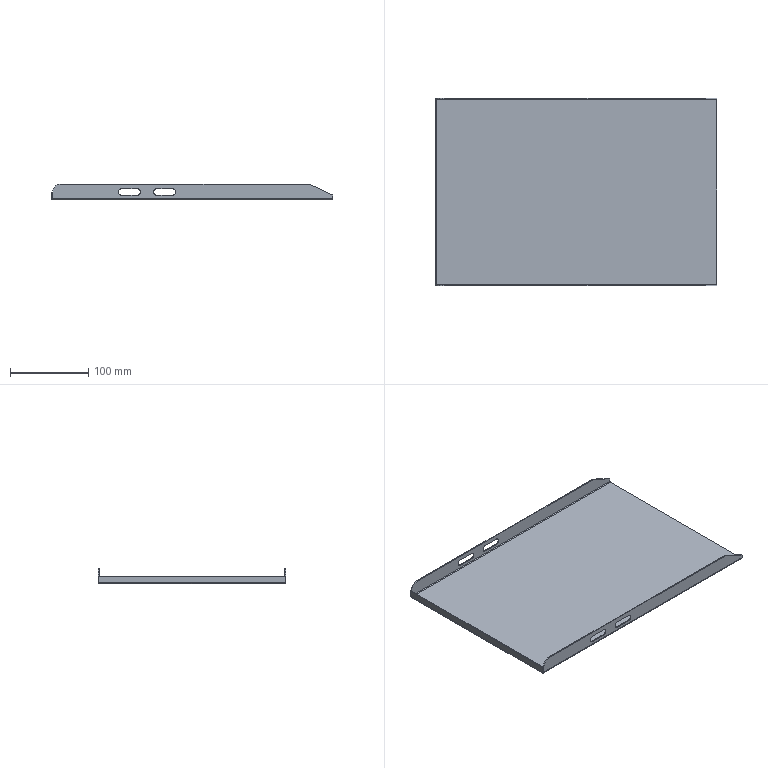Part | 1 solid | 52 faces | box 360 x 240 x 20 mm | volume 120091 mm3 | plane 36 | cylinder 16 | commonest cylinder face diameters 8.4 x8 1.473 x3 3.873 x3 20 x2
STEP:
#1=CARTESIAN_POINT('',(-178.063,120.,0.));
#2=VERTEX_POINT('',#1);
#3=CARTESIAN_POINT('',(-178.063,119.854,0.));
#4=VERTEX_POINT('',#3);
#5=CARTESIAN_POINT('',(-178.063,120.,0.));
#6=DIRECTION('',(0.,-1.,0.));
#7=VECTOR('',#6,1000.);
#8=LINE('',#5,#7);
#9=EDGE_CURVE('',#2,#4,#8,.T.);
#10=ORIENTED_EDGE('',*,*,#9,.T.);
#11=CARTESIAN_POINT('',(-178.063,118.063,-1.2));
#12=VERTEX_POINT('',#11);
#13=CARTESIAN_POINT('',(-178.063,118.063,0.7366));
#14=DIRECTION('',(-1.,0.,0.));
#15=DIRECTION('',(0.,0.,1.));
#16=AXIS2_PLACEMENT_3D('',#13,#14,#15);
#17=CIRCLE('',#16,1.937);
#18=EDGE_CURVE('',#4,#12,#17,.T.);
#19=ORIENTED_EDGE('',*,*,#18,.T.);
#20=CARTESIAN_POINT('',(-178.063,120.,-1.2));
#21=VERTEX_POINT('',#20);
#22=CARTESIAN_POINT('',(-178.063,-120.,-1.2));
#23=DIRECTION('',(0.,-1.,0.));
#24=VECTOR('',#23,1000.);
#25=LINE('',#22,#24);
#26=EDGE_CURVE('',#21,#12,#25,.T.);
#27=ORIENTED_EDGE('',*,*,#26,.F.);
#28=CARTESIAN_POINT('',(-178.063,120.,0.));
#29=DIRECTION('',(0.,0.,-1.));
#30=VECTOR('',#29,1000.);
#31=LINE('',#28,#30);
#32=EDGE_CURVE('',#2,#21,#31,.T.);
#33=ORIENTED_EDGE('',*,*,#32,.F.);
#34=EDGE_LOOP('',(#10,#19,#27,#33));
#35=FACE_OUTER_BOUND('',#34,.T.);
#36=CARTESIAN_POINT('',(-178.063,120.,0.));
#37=DIRECTION('',(1.,0.,0.));
#38=DIRECTION('',(0.,0.,-1.));
#39=AXIS2_PLACEMENT_3D('',#36,#37,#38);
#40=PLANE('',#39);
#41=ADVANCED_FACE('',(#35),#40,.T.);
#42=CARTESIAN_POINT('',(-178.063,-120.,-1.2));
#43=VERTEX_POINT('',#42);
#44=CARTESIAN_POINT('',(-178.063,-118.063,-1.2));
#45=VERTEX_POINT('',#44);
#46=CARTESIAN_POINT('',(-178.063,-120.,-1.2));
#47=DIRECTION('',(0.,1.,0.));
#48=VECTOR('',#47,1000.);
#49=LINE('',#46,#48);
#50=EDGE_CURVE('',#43,#45,#49,.T.);
#51=ORIENTED_EDGE('',*,*,#50,.T.);
#52=CARTESIAN_POINT('',(-178.063,-119.854,0.));
#53=VERTEX_POINT('',#52);
#54=CARTESIAN_POINT('',(-178.063,-118.063,0.7366));
#55=DIRECTION('',(-1.,0.,0.));
#56=DIRECTION('',(0.,0.,-1.));
#57=AXIS2_PLACEMENT_3D('',#54,#55,#56);
#58=CIRCLE('',#57,1.937);
#59=EDGE_CURVE('',#45,#53,#58,.T.);
#60=ORIENTED_EDGE('',*,*,#59,.T.);
#61=CARTESIAN_POINT('',(-178.063,-120.,0.));
#62=VERTEX_POINT('',#61);
#63=CARTESIAN_POINT('',(-178.063,-120.,0.));
#64=DIRECTION('',(0.,1.,0.));
#65=VECTOR('',#64,1000.);
#66=LINE('',#63,#65);
#67=EDGE_CURVE('',#62,#53,#66,.T.);
#68=ORIENTED_EDGE('',*,*,#67,.F.);
#69=CARTESIAN_POINT('',(-178.063,-120.,0.));
#70=DIRECTION('',(0.,0.,-1.));
#71=VECTOR('',#70,1000.);
#72=LINE('',#69,#71);
#73=EDGE_CURVE('',#62,#43,#72,.T.);
#74=ORIENTED_EDGE('',*,*,#73,.T.);
#75=EDGE_LOOP('',(#51,#60,#68,#74));
#76=FACE_OUTER_BOUND('',#75,.T.);
#77=CARTESIAN_POINT('',(-178.063,-118.063,0.));
#78=DIRECTION('',(1.,0.,0.));
#79=DIRECTION('',(0.,0.,-1.));
#80=AXIS2_PLACEMENT_3D('',#77,#78,#79);
#81=PLANE('',#80);
#82=ADVANCED_FACE('',(#76),#81,.T.);
#83=CARTESIAN_POINT('',(-178.063,-120.,-1.2));
#84=DIRECTION('',(0.,1.,0.));
#85=VECTOR('',#84,1000.);
#86=LINE('',#83,#85);
#87=EDGE_CURVE('',#45,#12,#86,.T.);
#88=ORIENTED_EDGE('',*,*,#87,.T.);
#89=CARTESIAN_POINT('',(180.,118.063,-1.2));
#90=VERTEX_POINT('',#89);
#91=CARTESIAN_POINT('',(-178.063,118.063,-1.2));
#92=DIRECTION('',(1.,0.,0.));
#93=VECTOR('',#92,1000.);
#94=LINE('',#91,#93);
#95=EDGE_CURVE('',#12,#90,#94,.T.);
#96=ORIENTED_EDGE('',*,*,#95,.T.);
#97=CARTESIAN_POINT('',(180.,-118.063,-1.2));
#98=VERTEX_POINT('',#97);
#99=CARTESIAN_POINT('',(180.,-120.,-1.2));
#100=DIRECTION('',(0.,1.,0.));
#101=VECTOR('',#100,1000.);
#102=LINE('',#99,#101);
#103=EDGE_CURVE('',#98,#90,#102,.T.);
#104=ORIENTED_EDGE('',*,*,#103,.F.);
#105=CARTESIAN_POINT('',(180.,-118.063,-1.2));
#106=DIRECTION('',(-1.,0.,0.));
#107=VECTOR('',#106,1000.);
#108=LINE('',#105,#107);
#109=EDGE_CURVE('',#98,#45,#108,.T.);
#110=ORIENTED_EDGE('',*,*,#109,.T.);
#111=EDGE_LOOP('',(#88,#96,#104,#110));
#112=FACE_OUTER_BOUND('',#111,.T.);
#113=CARTESIAN_POINT('',(0.,0.,-1.2));
#114=DIRECTION('',(0.,0.,-1.));
#115=DIRECTION('',(-1.,0.,0.));
#116=AXIS2_PLACEMENT_3D('',#113,#114,#115);
#117=PLANE('',#116);
#118=ADVANCED_FACE('',(#112),#117,.T.);
#119=CARTESIAN_POINT('',(-178.063,118.063,0.));
#120=VERTEX_POINT('',#119);
#121=CARTESIAN_POINT('',(180.,118.063,0.));
#122=VERTEX_POINT('',#121);
#123=CARTESIAN_POINT('',(-178.063,118.063,0.));
#124=DIRECTION('',(1.,0.,0.));
#125=VECTOR('',#124,1000.);
#126=LINE('',#123,#125);
#127=EDGE_CURVE('',#120,#122,#126,.T.);
#128=ORIENTED_EDGE('',*,*,#127,.F.);
#129=CARTESIAN_POINT('',(-178.063,-118.063,0.));
#130=VERTEX_POINT('',#129);
#131=CARTESIAN_POINT('',(-178.063,-120.,0.));
#132=DIRECTION('',(0.,1.,0.));
#133=VECTOR('',#132,1000.);
#134=LINE('',#131,#133);
#135=EDGE_CURVE('',#130,#120,#134,.T.);
#136=ORIENTED_EDGE('',*,*,#135,.F.);
#137=CARTESIAN_POINT('',(180.,-118.063,0.));
#138=VERTEX_POINT('',#137);
#139=CARTESIAN_POINT('',(180.,-118.063,0.));
#140=DIRECTION('',(-1.,0.,0.));
#141=VECTOR('',#140,1000.);
#142=LINE('',#139,#141);
#143=EDGE_CURVE('',#138,#130,#142,.T.);
#144=ORIENTED_EDGE('',*,*,#143,.F.);
#145=CARTESIAN_POINT('',(180.,-120.,0.));
#146=DIRECTION('',(0.,1.,0.));
#147=VECTOR('',#146,1000.);
#148=LINE('',#145,#147);
#149=EDGE_CURVE('',#138,#122,#148,.T.);
#150=ORIENTED_EDGE('',*,*,#149,.T.);
#151=EDGE_LOOP('',(#128,#136,#144,#150));
#152=FACE_OUTER_BOUND('',#151,.T.);
#153=CARTESIAN_POINT('',(0.,0.,0.));
#154=DIRECTION('',(0.,0.,-1.));
#155=DIRECTION('',(-1.,0.,0.));
#156=AXIS2_PLACEMENT_3D('',#153,#154,#155);
#157=PLANE('',#156);
#158=ADVANCED_FACE('',(#152),#157,.F.);
#159=CARTESIAN_POINT('',(180.,118.063,0.));
#160=DIRECTION('',(0.,0.,-1.));
#161=VECTOR('',#160,1000.);
#162=LINE('',#159,#161);
#163=EDGE_CURVE('',#122,#90,#162,.T.);
#164=ORIENTED_EDGE('',*,*,#163,.F.);
#165=ORIENTED_EDGE('',*,*,#149,.F.);
#166=CARTESIAN_POINT('',(180.,-118.063,0.));
#167=DIRECTION('',(0.,0.,-1.));
#168=VECTOR('',#167,1000.);
#169=LINE('',#166,#168);
#170=EDGE_CURVE('',#138,#98,#169,.T.);
#171=ORIENTED_EDGE('',*,*,#170,.T.);
#172=ORIENTED_EDGE('',*,*,#103,.T.);
#173=EDGE_LOOP('',(#164,#165,#171,#172));
#174=FACE_OUTER_BOUND('',#173,.T.);
#175=CARTESIAN_POINT('',(180.,-120.,-1.2));
#176=DIRECTION('',(1.,0.,0.));
#177=DIRECTION('',(0.,0.,-1.));
#178=AXIS2_PLACEMENT_3D('',#175,#176,#177);
#179=PLANE('',#178);
#180=ADVANCED_FACE('',(#174),#179,.T.);
#181=CARTESIAN_POINT('',(-178.8,120.,0.7366));
#182=VERTEX_POINT('',#181);
#183=CARTESIAN_POINT('',(-180.,120.,0.7366));
#184=VERTEX_POINT('',#183);
#185=CARTESIAN_POINT('',(-180.,120.,0.7366));
#186=DIRECTION('',(-1.,0.,0.));
#187=VECTOR('',#186,1000.);
#188=LINE('',#185,#187);
#189=EDGE_CURVE('',#182,#184,#188,.T.);
#190=ORIENTED_EDGE('',*,*,#189,.F.);
#191=CARTESIAN_POINT('',(-178.063,120.,0.7366));
#192=DIRECTION('',(0.,1.,0.));
#193=DIRECTION('',(0.,0.,-1.));
#194=AXIS2_PLACEMENT_3D('',#191,#192,#193);
#195=CIRCLE('',#194,0.7366);
#196=EDGE_CURVE('',#2,#182,#195,.T.);
#197=ORIENTED_EDGE('',*,*,#196,.F.);
#198=ORIENTED_EDGE('',*,*,#32,.T.);
#199=CARTESIAN_POINT('',(-178.063,120.,0.7366));
#200=DIRECTION('',(0.,1.,0.));
#201=DIRECTION('',(0.,0.,-1.));
#202=AXIS2_PLACEMENT_3D('',#199,#200,#201);
#203=CIRCLE('',#202,1.937);
#204=EDGE_CURVE('',#21,#184,#203,.T.);
#205=ORIENTED_EDGE('',*,*,#204,.T.);
#206=EDGE_LOOP('',(#190,#197,#198,#205));
#207=FACE_OUTER_BOUND('',#206,.T.);
#208=CARTESIAN_POINT('',(-178.063,120.,0.7366));
#209=DIRECTION('',(0.,1.,0.));
#210=DIRECTION('',(0.,0.,1.));
#211=AXIS2_PLACEMENT_3D('',#208,#209,#210);
#212=PLANE('',#211);
#213=ADVANCED_FACE('',(#207),#212,.T.);
#214=CARTESIAN_POINT('',(-178.8,-120.,0.7366));
#215=VERTEX_POINT('',#214);
#216=CARTESIAN_POINT('',(-178.063,-120.,0.7366));
#217=DIRECTION('',(0.,-1.,0.));
#218=DIRECTION('',(0.,0.,-1.));
#219=AXIS2_PLACEMENT_3D('',#216,#217,#218);
#220=CIRCLE('',#219,0.7366);
#221=EDGE_CURVE('',#215,#62,#220,.T.);
#222=ORIENTED_EDGE('',*,*,#221,.F.);
#223=CARTESIAN_POINT('',(-180.,-120.,0.7366));
#224=VERTEX_POINT('',#223);
#225=CARTESIAN_POINT('',(-178.8,-120.,0.7366));
#226=DIRECTION('',(-1.,0.,0.));
#227=VECTOR('',#226,1000.);
#228=LINE('',#225,#227);
#229=EDGE_CURVE('',#215,#224,#228,.T.);
#230=ORIENTED_EDGE('',*,*,#229,.T.);
#231=CARTESIAN_POINT('',(-178.063,-120.,0.7366));
#232=DIRECTION('',(0.,-1.,0.));
#233=DIRECTION('',(0.,0.,-1.));
#234=AXIS2_PLACEMENT_3D('',#231,#232,#233);
#235=CIRCLE('',#234,1.937);
#236=EDGE_CURVE('',#224,#43,#235,.T.);
#237=ORIENTED_EDGE('',*,*,#236,.T.);
#238=ORIENTED_EDGE('',*,*,#73,.F.);
#239=EDGE_LOOP('',(#222,#230,#237,#238));
#240=FACE_OUTER_BOUND('',#239,.T.);
#241=CARTESIAN_POINT('',(-178.063,-120.,0.7366));
#242=DIRECTION('',(0.,1.,0.));
#243=DIRECTION('',(0.,0.,1.));
#244=AXIS2_PLACEMENT_3D('',#241,#242,#243);
#245=PLANE('',#244);
#246=ADVANCED_FACE('',(#240),#245,.F.);
#247=ORIENTED_EDGE('',*,*,#50,.F.);
#248=ORIENTED_EDGE('',*,*,#236,.F.);
#249=CARTESIAN_POINT('',(-180.,0.,0.7366));
#250=DIRECTION('',(0.,-1.,0.));
#251=VECTOR('',#250,1000.);
#252=LINE('',#249,#251);
#253=EDGE_CURVE('',#184,#224,#252,.T.);
#254=ORIENTED_EDGE('',*,*,#253,.F.);
#255=ORIENTED_EDGE('',*,*,#204,.F.);
#256=ORIENTED_EDGE('',*,*,#26,.T.);
#257=ORIENTED_EDGE('',*,*,#87,.F.);
#258=EDGE_LOOP('',(#247,#248,#254,#255,#256,#257));
#259=FACE_OUTER_BOUND('',#258,.T.);
#260=CARTESIAN_POINT('',(-178.063,-120.,0.7366));
#261=DIRECTION('',(0.,-1.,0.));
#262=DIRECTION('',(-1.,0.,0.));
#263=AXIS2_PLACEMENT_3D('',#260,#261,#262);
#264=CYLINDRICAL_SURFACE('',#263,1.937);
#265=ADVANCED_FACE('',(#259),#264,.T.);
#266=ORIENTED_EDGE('',*,*,#67,.T.);
#267=CARTESIAN_POINT('',(-178.063,-120.,0.));
#268=DIRECTION('',(0.,1.,0.));
#269=VECTOR('',#268,1000.);
#270=LINE('',#267,#269);
#271=EDGE_CURVE('',#53,#130,#270,.T.);
#272=ORIENTED_EDGE('',*,*,#271,.T.);
#273=ORIENTED_EDGE('',*,*,#135,.T.);
#274=CARTESIAN_POINT('',(-178.063,120.,0.));
#275=DIRECTION('',(0.,-1.,0.));
#276=VECTOR('',#275,1000.);
#277=LINE('',#274,#276);
#278=EDGE_CURVE('',#4,#120,#277,.T.);
#279=ORIENTED_EDGE('',*,*,#278,.F.);
#280=ORIENTED_EDGE('',*,*,#9,.F.);
#281=ORIENTED_EDGE('',*,*,#196,.T.);
#282=CARTESIAN_POINT('',(-178.8,120.,0.7366));
#283=DIRECTION('',(0.,-1.,0.));
#284=VECTOR('',#283,1000.);
#285=LINE('',#282,#284);
#286=EDGE_CURVE('',#182,#215,#285,.T.);
#287=ORIENTED_EDGE('',*,*,#286,.T.);
#288=ORIENTED_EDGE('',*,*,#221,.T.);
#289=EDGE_LOOP('',(#266,#272,#273,#279,#280,#281,#287,#288));
#290=FACE_OUTER_BOUND('',#289,.T.);
#291=CARTESIAN_POINT('',(-178.063,-120.,0.7366));
#292=DIRECTION('',(0.,-1.,0.));
#293=DIRECTION('',(-1.,0.,0.));
#294=AXIS2_PLACEMENT_3D('',#291,#292,#293);
#295=CYLINDRICAL_SURFACE('',#294,0.7366);
#296=ADVANCED_FACE('',(#290),#295,.F.);
#297=CARTESIAN_POINT('',(-180.,-120.,8.8));
#298=VERTEX_POINT('',#297);
#299=CARTESIAN_POINT('',(-180.,-120.,0.));
#300=DIRECTION('',(0.,0.,-1.));
#301=VECTOR('',#300,1000.);
#302=LINE('',#299,#301);
#303=EDGE_CURVE('',#298,#224,#302,.T.);
#304=ORIENTED_EDGE('',*,*,#303,.T.);
#305=ORIENTED_EDGE('',*,*,#229,.F.);
#306=CARTESIAN_POINT('',(-178.8,-120.,8.8));
#307=VERTEX_POINT('',#306);
#308=CARTESIAN_POINT('',(-178.8,-120.,0.));
#309=DIRECTION('',(0.,0.,-1.));
#310=VECTOR('',#309,1000.);
#311=LINE('',#308,#310);
#312=EDGE_CURVE('',#307,#215,#311,.T.);
#313=ORIENTED_EDGE('',*,*,#312,.F.);
#314=CARTESIAN_POINT('',(-180.,-120.,8.8));
#315=DIRECTION('',(1.,0.,0.));
#316=VECTOR('',#315,1000.);
#317=LINE('',#314,#316);
#318=EDGE_CURVE('',#298,#307,#317,.T.);
#319=ORIENTED_EDGE('',*,*,#318,.F.);
#320=EDGE_LOOP('',(#304,#305,#313,#319));
#321=FACE_OUTER_BOUND('',#320,.T.);
#322=CARTESIAN_POINT('',(-180.,-120.,0.));
#323=DIRECTION('',(0.,-1.,0.));
#324=DIRECTION('',(0.,0.,-1.));
#325=AXIS2_PLACEMENT_3D('',#322,#323,#324);
#326=PLANE('',#325);
#327=ADVANCED_FACE('',(#321),#326,.T.);
#328=CARTESIAN_POINT('',(-178.8,120.,8.8));
#329=VERTEX_POINT('',#328);
#330=CARTESIAN_POINT('',(-178.8,120.,0.));
#331=DIRECTION('',(0.,0.,1.));
#332=VECTOR('',#331,1000.);
#333=LINE('',#330,#332);
#334=EDGE_CURVE('',#182,#329,#333,.T.);
#335=ORIENTED_EDGE('',*,*,#334,.F.);
#336=ORIENTED_EDGE('',*,*,#189,.T.);
#337=CARTESIAN_POINT('',(-180.,120.,8.8));
#338=VERTEX_POINT('',#337);
#339=CARTESIAN_POINT('',(-180.,120.,8.8));
#340=DIRECTION('',(0.,0.,1.));
#341=VECTOR('',#340,1000.);
#342=LINE('',#339,#341);
#343=EDGE_CURVE('',#184,#338,#342,.T.);
#344=ORIENTED_EDGE('',*,*,#343,.T.);
#345=CARTESIAN_POINT('',(-180.,120.,8.8));
#346=DIRECTION('',(1.,0.,0.));
#347=VECTOR('',#346,1000.);
#348=LINE('',#345,#347);
#349=EDGE_CURVE('',#338,#329,#348,.T.);
#350=ORIENTED_EDGE('',*,*,#349,.T.);
#351=EDGE_LOOP('',(#335,#336,#344,#350));
#352=FACE_OUTER_BOUND('',#351,.T.);
#353=CARTESIAN_POINT('',(-180.,120.,8.8));
#354=DIRECTION('',(0.,1.,0.));
#355=DIRECTION('',(0.,0.,1.));
#356=AXIS2_PLACEMENT_3D('',#353,#354,#355);
#357=PLANE('',#356);
#358=ADVANCED_FACE('',(#352),#357,.T.);
#359=ORIENTED_EDGE('',*,*,#343,.F.);
#360=ORIENTED_EDGE('',*,*,#253,.T.);
#361=ORIENTED_EDGE('',*,*,#303,.F.);
#362=CARTESIAN_POINT('',(-180.,-120.,8.8));
#363=DIRECTION('',(0.,-1.,0.));
#364=VECTOR('',#363,1000.);
#365=LINE('',#362,#364);
#366=EDGE_CURVE('',#338,#298,#365,.T.);
#367=ORIENTED_EDGE('',*,*,#366,.F.);
#368=EDGE_LOOP('',(#359,#360,#361,#367));
#369=FACE_OUTER_BOUND('',#368,.T.);
#370=CARTESIAN_POINT('',(-180.,0.,0.));
#371=DIRECTION('',(-1.,0.,0.));
#372=DIRECTION('',(0.,0.,1.));
#373=AXIS2_PLACEMENT_3D('',#370,#371,#372);
#374=PLANE('',#373);
#375=ADVANCED_FACE('',(#369),#374,.T.);
#376=ORIENTED_EDGE('',*,*,#286,.F.);
#377=ORIENTED_EDGE('',*,*,#334,.T.);
#378=CARTESIAN_POINT('',(-178.8,0.,8.8));
#379=DIRECTION('',(0.,-1.,0.));
#380=VECTOR('',#379,1000.);
#381=LINE('',#378,#380);
#382=EDGE_CURVE('',#329,#307,#381,.T.);
#383=ORIENTED_EDGE('',*,*,#382,.T.);
#384=ORIENTED_EDGE('',*,*,#312,.T.);
#385=EDGE_LOOP('',(#376,#377,#383,#384));
#386=FACE_OUTER_BOUND('',#385,.T.);
#387=CARTESIAN_POINT('',(-178.8,0.,0.));
#388=DIRECTION('',(-1.,0.,0.));
#389=DIRECTION('',(0.,0.,1.));
#390=AXIS2_PLACEMENT_3D('',#387,#388,#389);
#391=PLANE('',#390);
#392=ADVANCED_FACE('',(#386),#391,.F.);
#393=ORIENTED_EDGE('',*,*,#382,.F.);
#394=ORIENTED_EDGE('',*,*,#349,.F.);
#395=ORIENTED_EDGE('',*,*,#366,.T.);
#396=ORIENTED_EDGE('',*,*,#318,.T.);
#397=EDGE_LOOP('',(#393,#394,#395,#396));
#398=FACE_OUTER_BOUND('',#397,.T.);
#399=CARTESIAN_POINT('',(-180.,-120.,8.8));
#400=DIRECTION('',(0.,0.,1.));
#401=DIRECTION('',(1.,0.,0.));
#402=AXIS2_PLACEMENT_3D('',#399,#400,#401);
#403=PLANE('',#402);
#404=ADVANCED_FACE('',(#398),#403,.T.);
#405=ORIENTED_EDGE('',*,*,#271,.F.);
#406=CARTESIAN_POINT('',(-178.063,-120.,0.7366));
#407=VERTEX_POINT('',#406);
#408=CARTESIAN_POINT('',(-178.063,-118.063,0.7366));
#409=DIRECTION('',(-1.,0.,0.));
#410=DIRECTION('',(0.,0.,-1.));
#411=AXIS2_PLACEMENT_3D('',#408,#409,#410);
#412=CIRCLE('',#411,1.937);
#413=EDGE_CURVE('',#53,#407,#412,.T.);
#414=ORIENTED_EDGE('',*,*,#413,.T.);
#415=CARTESIAN_POINT('',(-178.063,-118.8,0.7366));
#416=VERTEX_POINT('',#415);
#417=CARTESIAN_POINT('',(-178.063,-120.,0.7366));
#418=DIRECTION('',(0.,-1.,0.));
#419=VECTOR('',#418,1000.);
#420=LINE('',#417,#419);
#421=EDGE_CURVE('',#416,#407,#420,.T.);
#422=ORIENTED_EDGE('',*,*,#421,.F.);
#423=CARTESIAN_POINT('',(-178.063,-118.063,0.7366));
#424=DIRECTION('',(-1.,0.,0.));
#425=DIRECTION('',(0.,0.,-1.));
#426=AXIS2_PLACEMENT_3D('',#423,#424,#425);
#427=CIRCLE('',#426,0.7366);
#428=EDGE_CURVE('',#130,#416,#427,.T.);
#429=ORIENTED_EDGE('',*,*,#428,.F.);
#430=EDGE_LOOP('',(#405,#414,#422,#429));
#431=FACE_OUTER_BOUND('',#430,.T.);
#432=CARTESIAN_POINT('',(-178.063,-118.063,0.7366));
#433=DIRECTION('',(-1.,0.,0.));
#434=DIRECTION('',(0.,0.,1.));
#435=AXIS2_PLACEMENT_3D('',#432,#433,#434);
#436=PLANE('',#435);
#437=ADVANCED_FACE('',(#431),#436,.T.);
#438=CARTESIAN_POINT('',(180.,-118.8,0.7366));
#439=VERTEX_POINT('',#438);
#440=CARTESIAN_POINT('',(180.,-118.063,0.7366));
#441=DIRECTION('',(1.,0.,0.));
#442=DIRECTION('',(0.,0.,-1.));
#443=AXIS2_PLACEMENT_3D('',#440,#441,#442);
#444=CIRCLE('',#443,0.7366);
#445=EDGE_CURVE('',#439,#138,#444,.T.);
#446=ORIENTED_EDGE('',*,*,#445,.F.);
#447=CARTESIAN_POINT('',(180.,-120.,0.7366));
#448=VERTEX_POINT('',#447);
#449=CARTESIAN_POINT('',(180.,-118.8,0.7366));
#450=DIRECTION('',(0.,-1.,0.));
#451=VECTOR('',#450,1000.);
#452=LINE('',#449,#451);
#453=EDGE_CURVE('',#439,#448,#452,.T.);
#454=ORIENTED_EDGE('',*,*,#453,.T.);
#455=CARTESIAN_POINT('',(180.,-118.063,0.7366));
#456=DIRECTION('',(1.,0.,0.));
#457=DIRECTION('',(0.,0.,-1.));
#458=AXIS2_PLACEMENT_3D('',#455,#456,#457);
#459=CIRCLE('',#458,1.937);
#460=EDGE_CURVE('',#448,#98,#459,.T.);
#461=ORIENTED_EDGE('',*,*,#460,.T.);
#462=ORIENTED_EDGE('',*,*,#170,.F.);
#463=EDGE_LOOP('',(#446,#454,#461,#462));
#464=FACE_OUTER_BOUND('',#463,.T.);
#465=CARTESIAN_POINT('',(180.,-118.063,0.7366));
#466=DIRECTION('',(-1.,0.,0.));
#467=DIRECTION('',(0.,0.,1.));
#468=AXIS2_PLACEMENT_3D('',#465,#466,#467);
#469=PLANE('',#468);
#470=ADVANCED_FACE('',(#464),#469,.F.);
#471=ORIENTED_EDGE('',*,*,#109,.F.);
#472=ORIENTED_EDGE('',*,*,#460,.F.);
#473=CARTESIAN_POINT('',(0.,-120.,0.7366));
#474=DIRECTION('',(1.,0.,0.));
#475=VECTOR('',#474,1000.);
#476=LINE('',#473,#475);
#477=EDGE_CURVE('',#407,#448,#476,.T.);
#478=ORIENTED_EDGE('',*,*,#477,.F.);
#479=ORIENTED_EDGE('',*,*,#413,.F.);
#480=ORIENTED_EDGE('',*,*,#59,.F.);
#481=EDGE_LOOP('',(#471,#472,#478,#479,#480));
#482=FACE_OUTER_BOUND('',#481,.T.);
#483=CARTESIAN_POINT('',(180.,-118.063,0.7366));
#484=DIRECTION('',(1.,0.,0.));
#485=DIRECTION('',(0.,-1.,0.));
#486=AXIS2_PLACEMENT_3D('',#483,#484,#485);
#487=CYLINDRICAL_SURFACE('',#486,1.937);
#488=ADVANCED_FACE('',(#482),#487,.T.);
#489=ORIENTED_EDGE('',*,*,#143,.T.);
#490=ORIENTED_EDGE('',*,*,#428,.T.);
#491=CARTESIAN_POINT('',(-178.063,-118.8,0.7366));
#492=DIRECTION('',(1.,0.,0.));
#493=VECTOR('',#492,1000.);
#494=LINE('',#491,#493);
#495=EDGE_CURVE('',#416,#439,#494,.T.);
#496=ORIENTED_EDGE('',*,*,#495,.T.);
#497=ORIENTED_EDGE('',*,*,#445,.T.);
#498=EDGE_LOOP('',(#489,#490,#496,#497));
#499=FACE_OUTER_BOUND('',#498,.T.);
#500=CARTESIAN_POINT('',(180.,-118.063,0.7366));
#501=DIRECTION('',(1.,0.,0.));
#502=DIRECTION('',(0.,-1.,0.));
#503=AXIS2_PLACEMENT_3D('',#500,#501,#502);
#504=CYLINDRICAL_SURFACE('',#503,0.7366);
#505=ADVANCED_FACE('',(#499),#504,.F.);
#506=CARTESIAN_POINT('',(180.,-118.8,5.));
#507=VERTEX_POINT('',#506);
#508=CARTESIAN_POINT('',(180.,-118.8,0.));
#509=DIRECTION('',(0.,0.,-1.));
#510=VECTOR('',#509,1000.);
#511=LINE('',#508,#510);
#512=EDGE_CURVE('',#507,#439,#511,.T.);
#513=ORIENTED_EDGE('',*,*,#512,.F.);
#514=CARTESIAN_POINT('',(180.,-120.,5.));
#515=VERTEX_POINT('',#514);
#516=CARTESIAN_POINT('',(180.,-120.,5.));
#517=DIRECTION('',(0.,-1.,0.));
#518=VECTOR('',#517,1000.);
#519=LINE('',#516,#518);
#520=EDGE_CURVE('',#507,#515,#519,.T.);
#521=ORIENTED_EDGE('',*,*,#520,.T.);
#522=CARTESIAN_POINT('',(180.,-120.,0.));
#523=DIRECTION('',(0.,0.,-1.));
#524=VECTOR('',#523,1000.);
#525=LINE('',#522,#524);
#526=EDGE_CURVE('',#515,#448,#525,.T.);
#527=ORIENTED_EDGE('',*,*,#526,.T.);
#528=ORIENTED_EDGE('',*,*,#453,.F.);
#529=EDGE_LOOP('',(#513,#521,#527,#528));
#530=FACE_OUTER_BOUND('',#529,.T.);
#531=CARTESIAN_POINT('',(180.,-120.,0.));
#532=DIRECTION('',(1.,0.,0.));
#533=DIRECTION('',(0.,1.,0.));
#534=AXIS2_PLACEMENT_3D('',#531,#532,#533);
#535=PLANE('',#534);
#536=ADVANCED_FACE('',(#530),#535,.T.);
#537=CARTESIAN_POINT('',(-178.063,-120.,8.8));
#538=VERTEX_POINT('',#537);
#539=CARTESIAN_POINT('',(-178.063,-120.,18.8));
#540=DIRECTION('',(0.,0.,1.));
#541=VECTOR('',#540,1000.);
#542=LINE('',#539,#541);
#543=EDGE_CURVE('',#407,#538,#542,.T.);
#544=ORIENTED_EDGE('',*,*,#543,.T.);
#545=CARTESIAN_POINT('',(-178.063,-118.8,8.8));
#546=VERTEX_POINT('',#545);
#547=CARTESIAN_POINT('',(-178.063,-120.,8.8));
#548=DIRECTION('',(0.,1.,0.));
#549=VECTOR('',#548,1000.);
#550=LINE('',#547,#549);
#551=EDGE_CURVE('',#538,#546,#550,.T.);
#552=ORIENTED_EDGE('',*,*,#551,.T.);
#553=CARTESIAN_POINT('',(-178.063,-118.8,0.));
#554=DIRECTION('',(0.,0.,1.));
#555=VECTOR('',#554,1000.);
#556=LINE('',#553,#555);
#557=EDGE_CURVE('',#416,#546,#556,.T.);
#558=ORIENTED_EDGE('',*,*,#557,.F.);
#559=ORIENTED_EDGE('',*,*,#421,.T.);
#560=EDGE_LOOP('',(#544,#552,#558,#559));
#561=FACE_OUTER_BOUND('',#560,.T.);
#562=CARTESIAN_POINT('',(-178.063,-120.,18.8));
#563=DIRECTION('',(-1.,0.,0.));
#564=DIRECTION('',(0.,-1.,0.));
#565=AXIS2_PLACEMENT_3D('',#562,#563,#564);
#566=PLANE('',#565);
#567=ADVANCED_FACE('',(#561),#566,.T.);
#568=CARTESIAN_POINT('',(-90.,-120.,13.));
#569=VERTEX_POINT('',#568);
#570=CARTESIAN_POINT('',(-90.,-120.,4.6));
#571=VERTEX_POINT('',#570);
#572=CARTESIAN_POINT('',(-90.,-120.,8.8));
#573=DIRECTION('',(0.,-1.,0.));
#574=DIRECTION('',(0.,0.,-1.));
#575=AXIS2_PLACEMENT_3D('',#572,#573,#574);
#576=CIRCLE('',#575,4.2);
#577=EDGE_CURVE('',#569,#571,#576,.T.);
#578=ORIENTED_EDGE('',*,*,#577,.F.);
#579=CARTESIAN_POINT('',(-70.,-120.,13.));
#580=VERTEX_POINT('',#579);
#581=CARTESIAN_POINT('',(-90.,-120.,13.));
#582=DIRECTION('',(-1.,0.,0.));
#583=VECTOR('',#582,1000.);
#584=LINE('',#581,#583);
#585=EDGE_CURVE('',#580,#569,#584,.T.);
#586=ORIENTED_EDGE('',*,*,#585,.F.);
#587=CARTESIAN_POINT('',(-70.,-120.,4.6));
#588=VERTEX_POINT('',#587);
#589=CARTESIAN_POINT('',(-70.,-120.,8.8));
#590=DIRECTION('',(0.,-1.,0.));
#591=DIRECTION('',(0.,0.,-1.));
#592=AXIS2_PLACEMENT_3D('',#589,#590,#591);
#593=CIRCLE('',#592,4.2);
#594=EDGE_CURVE('',#588,#580,#593,.T.);
#595=ORIENTED_EDGE('',*,*,#594,.F.);
#596=CARTESIAN_POINT('',(-90.,-120.,4.6));
#597=DIRECTION('',(1.,0.,0.));
#598=VECTOR('',#597,1000.);
#599=LINE('',#596,#598);
#600=EDGE_CURVE('',#571,#588,#599,.T.);
#601=ORIENTED_EDGE('',*,*,#600,.F.);
#602=EDGE_LOOP('',(#578,#586,#595,#601));
#603=FACE_BOUND('',#602,.T.);
#604=CARTESIAN_POINT('',(-45.,-120.,13.));
#605=VERTEX_POINT('',#604);
#606=CARTESIAN_POINT('',(-45.,-120.,4.6));
#607=VERTEX_POINT('',#606);
#608=CARTESIAN_POINT('',(-45.,-120.,8.8));
#609=DIRECTION('',(0.,-1.,0.));
#610=DIRECTION('',(0.,0.,-1.));
#611=AXIS2_PLACEMENT_3D('',#608,#609,#610);
#612=CIRCLE('',#611,4.2);
#613=EDGE_CURVE('',#605,#607,#612,.T.);
#614=ORIENTED_EDGE('',*,*,#613,.F.);
#615=CARTESIAN_POINT('',(-25.,-120.,13.));
#616=VERTEX_POINT('',#615);
#617=CARTESIAN_POINT('',(-45.,-120.,13.));
#618=DIRECTION('',(-1.,0.,0.));
#619=VECTOR('',#618,1000.);
#620=LINE('',#617,#619);
#621=EDGE_CURVE('',#616,#605,#620,.T.);
#622=ORIENTED_EDGE('',*,*,#621,.F.);
#623=CARTESIAN_POINT('',(-25.,-120.,4.6));
#624=VERTEX_POINT('',#623);
#625=CARTESIAN_POINT('',(-25.,-120.,8.8));
#626=DIRECTION('',(0.,-1.,0.));
#627=DIRECTION('',(0.,0.,-1.));
#628=AXIS2_PLACEMENT_3D('',#625,#626,#627);
#629=CIRCLE('',#628,4.2);
#630=EDGE_CURVE('',#624,#616,#629,.T.);
#631=ORIENTED_EDGE('',*,*,#630,.F.);
#632=CARTESIAN_POINT('',(-45.,-120.,4.6));
#633=DIRECTION('',(1.,0.,0.));
#634=VECTOR('',#633,1000.);
#635=LINE('',#632,#634);
#636=EDGE_CURVE('',#607,#624,#635,.T.);
#637=ORIENTED_EDGE('',*,*,#636,.F.);
#638=EDGE_LOOP('',(#614,#622,#631,#637));
#639=FACE_BOUND('',#638,.T.);
#640=ORIENTED_EDGE('',*,*,#526,.F.);
#641=CARTESIAN_POINT('',(150.,-120.,18.8));
#642=VERTEX_POINT('',#641);
#643=CARTESIAN_POINT('',(33.334,-120.,72.466));
#644=DIRECTION('',(-0.9085,0.,0.4179));
#645=VECTOR('',#644,1000.);
#646=LINE('',#643,#645);
#647=EDGE_CURVE('',#515,#642,#646,.T.);
#648=ORIENTED_EDGE('',*,*,#647,.T.);
#649=CARTESIAN_POINT('',(-168.063,-120.,18.8));
#650=VERTEX_POINT('',#649);
#651=CARTESIAN_POINT('',(180.,-120.,18.8));
#652=DIRECTION('',(1.,0.,0.));
#653=VECTOR('',#652,1000.);
#654=LINE('',#651,#653);
#655=EDGE_CURVE('',#650,#642,#654,.T.);
#656=ORIENTED_EDGE('',*,*,#655,.F.);
#657=CARTESIAN_POINT('',(-168.063,-120.,8.8));
#658=DIRECTION('',(0.,-1.,0.));
#659=DIRECTION('',(0.,0.,-1.));
#660=AXIS2_PLACEMENT_3D('',#657,#658,#659);
#661=CIRCLE('',#660,10.);
#662=EDGE_CURVE('',#650,#538,#661,.T.);
#663=ORIENTED_EDGE('',*,*,#662,.T.);
#664=ORIENTED_EDGE('',*,*,#543,.F.);
#665=ORIENTED_EDGE('',*,*,#477,.T.);
#666=EDGE_LOOP('',(#640,#648,#656,#663,#664,#665));
#667=FACE_OUTER_BOUND('',#666,.T.);
#668=CARTESIAN_POINT('',(0.,-120.,0.));
#669=DIRECTION('',(0.,-1.,0.));
#670=DIRECTION('',(0.,0.,-1.));
#671=AXIS2_PLACEMENT_3D('',#668,#669,#670);
#672=PLANE('',#671);
#673=ADVANCED_FACE('',(#603,#639,#667),#672,.T.);
#674=CARTESIAN_POINT('',(-70.,-118.8,13.));
#675=VERTEX_POINT('',#674);
#676=CARTESIAN_POINT('',(-90.,-118.8,13.));
#677=VERTEX_POINT('',#676);
#678=CARTESIAN_POINT('',(0.,-118.8,13.));
#679=DIRECTION('',(-1.,0.,0.));
#680=VECTOR('',#679,1000.);
#681=LINE('',#678,#680);
#682=EDGE_CURVE('',#675,#677,#681,.T.);
#683=ORIENTED_EDGE('',*,*,#682,.T.);
#684=CARTESIAN_POINT('',(-90.,-118.8,4.6));
#685=VERTEX_POINT('',#684);
#686=CARTESIAN_POINT('',(-90.,-118.8,8.8));
#687=DIRECTION('',(0.,-1.,0.));
#688=DIRECTION('',(0.,0.,-1.));
#689=AXIS2_PLACEMENT_3D('',#686,#687,#688);
#690=CIRCLE('',#689,4.2);
#691=EDGE_CURVE('',#677,#685,#690,.T.);
#692=ORIENTED_EDGE('',*,*,#691,.T.);
#693=CARTESIAN_POINT('',(-70.,-118.8,4.6));
#694=VERTEX_POINT('',#693);
#695=CARTESIAN_POINT('',(0.,-118.8,4.6));
#696=DIRECTION('',(1.,0.,0.));
#697=VECTOR('',#696,1000.);
#698=LINE('',#695,#697);
#699=EDGE_CURVE('',#685,#694,#698,.T.);
#700=ORIENTED_EDGE('',*,*,#699,.T.);
#701=CARTESIAN_POINT('',(-70.,-118.8,8.8));
#702=DIRECTION('',(0.,-1.,0.));
#703=DIRECTION('',(0.,0.,-1.));
#704=AXIS2_PLACEMENT_3D('',#701,#702,#703);
#705=CIRCLE('',#704,4.2);
#706=EDGE_CURVE('',#694,#675,#705,.T.);
#707=ORIENTED_EDGE('',*,*,#706,.T.);
#708=EDGE_LOOP('',(#683,#692,#700,#707));
#709=FACE_BOUND('',#708,.T.);
#710=CARTESIAN_POINT('',(-25.,-118.8,13.));
#711=VERTEX_POINT('',#710);
#712=CARTESIAN_POINT('',(-45.,-118.8,13.));
#713=VERTEX_POINT('',#712);
#714=CARTESIAN_POINT('',(0.,-118.8,13.));
#715=DIRECTION('',(-1.,0.,0.));
#716=VECTOR('',#715,1000.);
#717=LINE('',#714,#716);
#718=EDGE_CURVE('',#711,#713,#717,.T.);
#719=ORIENTED_EDGE('',*,*,#718,.T.);
#720=CARTESIAN_POINT('',(-45.,-118.8,4.6));
#721=VERTEX_POINT('',#720);
#722=CARTESIAN_POINT('',(-45.,-118.8,8.8));
#723=DIRECTION('',(0.,-1.,0.));
#724=DIRECTION('',(0.,0.,-1.));
#725=AXIS2_PLACEMENT_3D('',#722,#723,#724);
#726=CIRCLE('',#725,4.2);
#727=EDGE_CURVE('',#713,#721,#726,.T.);
#728=ORIENTED_EDGE('',*,*,#727,.T.);
#729=CARTESIAN_POINT('',(-25.,-118.8,4.6));
#730=VERTEX_POINT('',#729);
#731=CARTESIAN_POINT('',(0.,-118.8,4.6));
#732=DIRECTION('',(1.,0.,0.));
#733=VECTOR('',#732,1000.);
#734=LINE('',#731,#733);
#735=EDGE_CURVE('',#721,#730,#734,.T.);
#736=ORIENTED_EDGE('',*,*,#735,.T.);
#737=CARTESIAN_POINT('',(-25.,-118.8,8.8));
#738=DIRECTION('',(0.,-1.,0.));
#739=DIRECTION('',(0.,0.,-1.));
#740=AXIS2_PLACEMENT_3D('',#737,#738,#739);
#741=CIRCLE('',#740,4.2);
#742=EDGE_CURVE('',#730,#711,#741,.T.);
#743=ORIENTED_EDGE('',*,*,#742,.T.);
#744=EDGE_LOOP('',(#719,#728,#736,#743));
#745=FACE_BOUND('',#744,.T.);
#746=CARTESIAN_POINT('',(-168.063,-118.8,18.8));
#747=VERTEX_POINT('',#746);
#748=CARTESIAN_POINT('',(150.,-118.8,18.8));
#749=VERTEX_POINT('',#748);
#750=CARTESIAN_POINT('',(0.,-118.8,18.8));
#751=DIRECTION('',(1.,0.,0.));
#752=VECTOR('',#751,1000.);
#753=LINE('',#750,#752);
#754=EDGE_CURVE('',#747,#749,#753,.T.);
#755=ORIENTED_EDGE('',*,*,#754,.T.);
#756=CARTESIAN_POINT('',(150.,-118.8,18.8));
#757=DIRECTION('',(0.9085,0.,-0.4179));
#758=VECTOR('',#757,1000.);
#759=LINE('',#756,#758);
#760=EDGE_CURVE('',#749,#507,#759,.T.);
#761=ORIENTED_EDGE('',*,*,#760,.T.);
#762=ORIENTED_EDGE('',*,*,#512,.T.);
#763=ORIENTED_EDGE('',*,*,#495,.F.);
#764=ORIENTED_EDGE('',*,*,#557,.T.);
#765=CARTESIAN_POINT('',(-168.063,-118.8,8.8));
#766=DIRECTION('',(0.,1.,0.));
#767=DIRECTION('',(0.,0.,-1.));
#768=AXIS2_PLACEMENT_3D('',#765,#766,#767);
#769=CIRCLE('',#768,10.);
#770=EDGE_CURVE('',#546,#747,#769,.T.);
#771=ORIENTED_EDGE('',*,*,#770,.T.);
#772=EDGE_LOOP('',(#755,#761,#762,#763,#764,#771));
#773=FACE_OUTER_BOUND('',#772,.T.);
#774=CARTESIAN_POINT('',(0.,-118.8,0.));
#775=DIRECTION('',(0.,-1.,0.));
#776=DIRECTION('',(0.,0.,-1.));
#777=AXIS2_PLACEMENT_3D('',#774,#775,#776);
#778=PLANE('',#777);
#779=ADVANCED_FACE('',(#709,#745,#773),#778,.F.);
#780=ORIENTED_EDGE('',*,*,#655,.T.);
#781=CARTESIAN_POINT('',(150.,-120.,18.8));
#782=DIRECTION('',(0.,1.,0.));
#783=VECTOR('',#782,1000.);
#784=LINE('',#781,#783);
#785=EDGE_CURVE('',#642,#749,#784,.T.);
#786=ORIENTED_EDGE('',*,*,#785,.T.);
#787=ORIENTED_EDGE('',*,*,#754,.F.);
#788=CARTESIAN_POINT('',(-168.063,-120.,18.8));
#789=DIRECTION('',(0.,-1.,0.));
#790=VECTOR('',#789,1000.);
#791=LINE('',#788,#790);
#792=EDGE_CURVE('',#747,#650,#791,.T.);
#793=ORIENTED_EDGE('',*,*,#792,.T.);
#794=EDGE_LOOP('',(#780,#786,#787,#793));
#795=FACE_OUTER_BOUND('',#794,.T.);
#796=CARTESIAN_POINT('',(180.,-120.,18.8));
#797=DIRECTION('',(0.,0.,1.));
#798=DIRECTION('',(0.,-1.,0.));
#799=AXIS2_PLACEMENT_3D('',#796,#797,#798);
#800=PLANE('',#799);
#801=ADVANCED_FACE('',(#795),#800,.T.);
#802=CARTESIAN_POINT('',(180.,118.8,0.7366));
#803=VERTEX_POINT('',#802);
#804=CARTESIAN_POINT('',(180.,120.,0.7366));
#805=VERTEX_POINT('',#804);
#806=CARTESIAN_POINT('',(180.,120.,0.7366));
#807=DIRECTION('',(0.,1.,0.));
#808=VECTOR('',#807,1000.);
#809=LINE('',#806,#808);
#810=EDGE_CURVE('',#803,#805,#809,.T.);
#811=ORIENTED_EDGE('',*,*,#810,.F.);
#812=CARTESIAN_POINT('',(180.,118.063,0.7366));
#813=DIRECTION('',(1.,0.,0.));
#814=DIRECTION('',(0.,0.,1.));
#815=AXIS2_PLACEMENT_3D('',#812,#813,#814);
#816=CIRCLE('',#815,0.7366);
#817=EDGE_CURVE('',#122,#803,#816,.T.);
#818=ORIENTED_EDGE('',*,*,#817,.F.);
#819=ORIENTED_EDGE('',*,*,#163,.T.);
#820=CARTESIAN_POINT('',(180.,118.063,0.7366));
#821=DIRECTION('',(1.,0.,0.));
#822=DIRECTION('',(0.,0.,1.));
#823=AXIS2_PLACEMENT_3D('',#820,#821,#822);
#824=CIRCLE('',#823,1.937);
#825=EDGE_CURVE('',#90,#805,#824,.T.);
#826=ORIENTED_EDGE('',*,*,#825,.T.);
#827=EDGE_LOOP('',(#811,#818,#819,#826));
#828=FACE_OUTER_BOUND('',#827,.T.);
#829=CARTESIAN_POINT('',(180.,118.063,0.7366));
#830=DIRECTION('',(1.,0.,0.));
#831=DIRECTION('',(0.,0.,-1.));
#832=AXIS2_PLACEMENT_3D('',#829,#830,#831);
#833=PLANE('',#832);
#834=ADVANCED_FACE('',(#828),#833,.T.);
#835=CARTESIAN_POINT('',(-178.063,120.,0.7366));
#836=VERTEX_POINT('',#835);
#837=CARTESIAN_POINT('',(-178.063,118.063,0.7366));
#838=DIRECTION('',(-1.,0.,0.));
#839=DIRECTION('',(0.,0.,1.));
#840=AXIS2_PLACEMENT_3D('',#837,#838,#839);
#841=CIRCLE('',#840,1.937);
#842=EDGE_CURVE('',#836,#4,#841,.T.);
#843=ORIENTED_EDGE('',*,*,#842,.T.);
#844=ORIENTED_EDGE('',*,*,#278,.T.);
#845=CARTESIAN_POINT('',(-178.063,118.8,0.7366));
#846=VERTEX_POINT('',#845);
#847=CARTESIAN_POINT('',(-178.063,118.063,0.7366));
#848=DIRECTION('',(-1.,0.,0.));
#849=DIRECTION('',(0.,0.,1.));
#850=AXIS2_PLACEMENT_3D('',#847,#848,#849);
#851=CIRCLE('',#850,0.7366);
#852=EDGE_CURVE('',#846,#120,#851,.T.);
#853=ORIENTED_EDGE('',*,*,#852,.F.);
#854=CARTESIAN_POINT('',(-178.063,118.8,0.7366));
#855=DIRECTION('',(0.,1.,0.));
#856=VECTOR('',#855,1000.);
#857=LINE('',#854,#856);
#858=EDGE_CURVE('',#846,#836,#857,.T.);
#859=ORIENTED_EDGE('',*,*,#858,.T.);
#860=EDGE_LOOP('',(#843,#844,#853,#859));
#861=FACE_OUTER_BOUND('',#860,.T.);
#862=CARTESIAN_POINT('',(-178.063,118.063,0.7366));
#863=DIRECTION('',(1.,0.,0.));
#864=DIRECTION('',(0.,0.,-1.));
#865=AXIS2_PLACEMENT_3D('',#862,#863,#864);
#866=PLANE('',#865);
#867=ADVANCED_FACE('',(#861),#866,.F.);
#868=ORIENTED_EDGE('',*,*,#95,.F.);
#869=ORIENTED_EDGE('',*,*,#18,.F.);
#870=ORIENTED_EDGE('',*,*,#842,.F.);
#871=CARTESIAN_POINT('',(180.,120.,0.7366));
#872=DIRECTION('',(1.,0.,0.));
#873=VECTOR('',#872,1000.);
#874=LINE('',#871,#873);
#875=EDGE_CURVE('',#836,#805,#874,.T.);
#876=ORIENTED_EDGE('',*,*,#875,.T.);
#877=ORIENTED_EDGE('',*,*,#825,.F.);
#878=EDGE_LOOP('',(#868,#869,#870,#876,#877));
#879=FACE_OUTER_BOUND('',#878,.T.);
#880=CARTESIAN_POINT('',(-178.063,118.063,0.7366));
#881=DIRECTION('',(-1.,0.,0.));
#882=DIRECTION('',(0.,1.,0.));
#883=AXIS2_PLACEMENT_3D('',#880,#881,#882);
#884=CYLINDRICAL_SURFACE('',#883,1.937);
#885=ADVANCED_FACE('',(#879),#884,.T.);
#886=ORIENTED_EDGE('',*,*,#127,.T.);
#887=ORIENTED_EDGE('',*,*,#817,.T.);
#888=CARTESIAN_POINT('',(180.,118.8,0.7366));
#889=DIRECTION('',(-1.,0.,0.));
#890=VECTOR('',#889,1000.);
#891=LINE('',#888,#890);
#892=EDGE_CURVE('',#803,#846,#891,.T.);
#893=ORIENTED_EDGE('',*,*,#892,.T.);
#894=ORIENTED_EDGE('',*,*,#852,.T.);
#895=EDGE_LOOP('',(#886,#887,#893,#894));
#896=FACE_OUTER_BOUND('',#895,.T.);
#897=CARTESIAN_POINT('',(-178.063,118.063,0.7366));
#898=DIRECTION('',(-1.,0.,0.));
#899=DIRECTION('',(0.,1.,0.));
#900=AXIS2_PLACEMENT_3D('',#897,#898,#899);
#901=CYLINDRICAL_SURFACE('',#900,0.7366);
#902=ADVANCED_FACE('',(#896),#901,.F.);
#903=CARTESIAN_POINT('',(180.,120.,5.));
#904=VERTEX_POINT('',#903);
#905=CARTESIAN_POINT('',(180.,120.,0.));
#906=DIRECTION('',(0.,0.,1.));
#907=VECTOR('',#906,1000.);
#908=LINE('',#905,#907);
#909=EDGE_CURVE('',#805,#904,#908,.T.);
#910=ORIENTED_EDGE('',*,*,#909,.T.);
#911=CARTESIAN_POINT('',(180.,118.8,5.));
#912=VERTEX_POINT('',#911);
#913=CARTESIAN_POINT('',(180.,120.,5.));
#914=DIRECTION('',(0.,-1.,0.));
#915=VECTOR('',#914,1000.);
#916=LINE('',#913,#915);
#917=EDGE_CURVE('',#904,#912,#916,.T.);
#918=ORIENTED_EDGE('',*,*,#917,.T.);
#919=CARTESIAN_POINT('',(180.,118.8,0.));
#920=DIRECTION('',(0.,0.,1.));
#921=VECTOR('',#920,1000.);
#922=LINE('',#919,#921);
#923=EDGE_CURVE('',#803,#912,#922,.T.);
#924=ORIENTED_EDGE('',*,*,#923,.F.);
#925=ORIENTED_EDGE('',*,*,#810,.T.);
#926=EDGE_LOOP('',(#910,#918,#924,#925));
#927=FACE_OUTER_BOUND('',#926,.T.);
#928=CARTESIAN_POINT('',(180.,120.,0.));
#929=DIRECTION('',(1.,0.,0.));
#930=DIRECTION('',(0.,1.,0.));
#931=AXIS2_PLACEMENT_3D('',#928,#929,#930);
#932=PLANE('',#931);
#933=ADVANCED_FACE('',(#927),#932,.T.);
#934=CARTESIAN_POINT('',(-178.063,118.8,8.8));
#935=VERTEX_POINT('',#934);
#936=CARTESIAN_POINT('',(-178.063,118.8,0.));
#937=DIRECTION('',(0.,0.,-1.));
#938=VECTOR('',#937,1000.);
#939=LINE('',#936,#938);
#940=EDGE_CURVE('',#935,#846,#939,.T.);
#941=ORIENTED_EDGE('',*,*,#940,.F.);
#942=CARTESIAN_POINT('',(-178.063,120.,8.8));
#943=VERTEX_POINT('',#942);
#944=CARTESIAN_POINT('',(-178.063,120.,8.8));
#945=DIRECTION('',(0.,1.,0.));
#946=VECTOR('',#945,1000.);
#947=LINE('',#944,#946);
#948=EDGE_CURVE('',#935,#943,#947,.T.);
#949=ORIENTED_EDGE('',*,*,#948,.T.);
#950=CARTESIAN_POINT('',(-178.063,120.,18.8));
#951=DIRECTION('',(0.,0.,-1.));
#952=VECTOR('',#951,1000.);
#953=LINE('',#950,#952);
#954=EDGE_CURVE('',#943,#836,#953,.T.);
#955=ORIENTED_EDGE('',*,*,#954,.T.);
#956=ORIENTED_EDGE('',*,*,#858,.F.);
#957=EDGE_LOOP('',(#941,#949,#955,#956));
#958=FACE_OUTER_BOUND('',#957,.T.);
#959=CARTESIAN_POINT('',(-178.063,120.,18.8));
#960=DIRECTION('',(-1.,0.,0.));
#961=DIRECTION('',(0.,-1.,0.));
#962=AXIS2_PLACEMENT_3D('',#959,#960,#961);
#963=PLANE('',#962);
#964=ADVANCED_FACE('',(#958),#963,.T.);
#965=CARTESIAN_POINT('',(-70.,120.,13.));
#966=VERTEX_POINT('',#965);
#967=CARTESIAN_POINT('',(-90.,120.,13.));
#968=VERTEX_POINT('',#967);
#969=CARTESIAN_POINT('',(-90.,120.,13.));
#970=DIRECTION('',(-1.,0.,0.));
#971=VECTOR('',#970,1000.);
#972=LINE('',#969,#971);
#973=EDGE_CURVE('',#966,#968,#972,.T.);
#974=ORIENTED_EDGE('',*,*,#973,.T.);
#975=CARTESIAN_POINT('',(-90.,120.,4.6));
#976=VERTEX_POINT('',#975);
#977=CARTESIAN_POINT('',(-90.,120.,8.8));
#978=DIRECTION('',(0.,-1.,0.));
#979=DIRECTION('',(0.,0.,-1.));
#980=AXIS2_PLACEMENT_3D('',#977,#978,#979);
#981=CIRCLE('',#980,4.2);
#982=EDGE_CURVE('',#968,#976,#981,.T.);
#983=ORIENTED_EDGE('',*,*,#982,.T.);
#984=CARTESIAN_POINT('',(-70.,120.,4.6));
#985=VERTEX_POINT('',#984);
#986=CARTESIAN_POINT('',(-90.,120.,4.6));
#987=DIRECTION('',(1.,0.,0.));
#988=VECTOR('',#987,1000.);
#989=LINE('',#986,#988);
#990=EDGE_CURVE('',#976,#985,#989,.T.);
#991=ORIENTED_EDGE('',*,*,#990,.T.);
#992=CARTESIAN_POINT('',(-70.,120.,8.8));
#993=DIRECTION('',(0.,-1.,0.));
#994=DIRECTION('',(0.,0.,-1.));
#995=AXIS2_PLACEMENT_3D('',#992,#993,#994);
#996=CIRCLE('',#995,4.2);
#997=EDGE_CURVE('',#985,#966,#996,.T.);
#998=ORIENTED_EDGE('',*,*,#997,.T.);
#999=EDGE_LOOP('',(#974,#983,#991,#998));
#1000=FACE_BOUND('',#999,.T.);
#1001=CARTESIAN_POINT('',(-25.,120.,13.));
#1002=VERTEX_POINT('',#1001);
#1003=CARTESIAN_POINT('',(-45.,120.,13.));
#1004=VERTEX_POINT('',#1003);
#1005=CARTESIAN_POINT('',(-45.,120.,13.));
#1006=DIRECTION('',(-1.,0.,0.));
#1007=VECTOR('',#1006,1000.);
#1008=LINE('',#1005,#1007);
#1009=EDGE_CURVE('',#1002,#1004,#1008,.T.);
#1010=ORIENTED_EDGE('',*,*,#1009,.T.);
#1011=CARTESIAN_POINT('',(-45.,120.,4.6));
#1012=VERTEX_POINT('',#1011);
#1013=CARTESIAN_POINT('',(-45.,120.,8.8));
#1014=DIRECTION('',(0.,-1.,0.));
#1015=DIRECTION('',(0.,0.,-1.));
#1016=AXIS2_PLACEMENT_3D('',#1013,#1014,#1015);
#1017=CIRCLE('',#1016,4.2);
#1018=EDGE_CURVE('',#1004,#1012,#1017,.T.);
#1019=ORIENTED_EDGE('',*,*,#1018,.T.);
#1020=CARTESIAN_POINT('',(-25.,120.,4.6));
#1021=VERTEX_POINT('',#1020);
#1022=CARTESIAN_POINT('',(-45.,120.,4.6));
#1023=DIRECTION('',(1.,0.,0.));
#1024=VECTOR('',#1023,1000.);
#1025=LINE('',#1022,#1024);
#1026=EDGE_CURVE('',#1012,#1021,#1025,.T.);
#1027=ORIENTED_EDGE('',*,*,#1026,.T.);
#1028=CARTESIAN_POINT('',(-25.,120.,8.8));
#1029=DIRECTION('',(0.,-1.,0.));
#1030=DIRECTION('',(0.,0.,-1.));
#1031=AXIS2_PLACEMENT_3D('',#1028,#1029,#1030);
#1032=CIRCLE('',#1031,4.2);
#1033=EDGE_CURVE('',#1021,#1002,#1032,.T.);
#1034=ORIENTED_EDGE('',*,*,#1033,.T.);
#1035=EDGE_LOOP('',(#1010,#1019,#1027,#1034));
#1036=FACE_BOUND('',#1035,.T.);
#1037=CARTESIAN_POINT('',(150.,120.,18.8));
#1038=VERTEX_POINT('',#1037);
#1039=CARTESIAN_POINT('',(-168.063,120.,18.8));
#1040=VERTEX_POINT('',#1039);
#1041=CARTESIAN_POINT('',(180.,120.,18.8));
#1042=DIRECTION('',(-1.,0.,0.));
#1043=VECTOR('',#1042,1000.);
#1044=LINE('',#1041,#1043);
#1045=EDGE_CURVE('',#1038,#1040,#1044,.T.);
#1046=ORIENTED_EDGE('',*,*,#1045,.F.);
#1047=CARTESIAN_POINT('',(180.,120.,5.));
#1048=DIRECTION('',(0.9085,0.,-0.4179));
#1049=VECTOR('',#1048,1000.);
#1050=LINE('',#1047,#1049);
#1051=EDGE_CURVE('',#1038,#904,#1050,.T.);
#1052=ORIENTED_EDGE('',*,*,#1051,.T.);
#1053=ORIENTED_EDGE('',*,*,#909,.F.);
#1054=ORIENTED_EDGE('',*,*,#875,.F.);
#1055=ORIENTED_EDGE('',*,*,#954,.F.);
#1056=CARTESIAN_POINT('',(-168.063,120.,8.8));
#1057=DIRECTION('',(0.,1.,0.));
#1058=DIRECTION('',(0.,0.,-1.));
#1059=AXIS2_PLACEMENT_3D('',#1056,#1057,#1058);
#1060=CIRCLE('',#1059,10.);
#1061=EDGE_CURVE('',#943,#1040,#1060,.T.);
#1062=ORIENTED_EDGE('',*,*,#1061,.T.);
#1063=EDGE_LOOP('',(#1046,#1052,#1053,#1054,#1055,#1062));
#1064=FACE_OUTER_BOUND('',#1063,.T.);
#1065=CARTESIAN_POINT('',(0.,120.,0.));
#1066=DIRECTION('',(0.,-1.,0.));
#1067=DIRECTION('',(0.,0.,-1.));
#1068=AXIS2_PLACEMENT_3D('',#1065,#1066,#1067);
#1069=PLANE('',#1068);
#1070=ADVANCED_FACE('',(#1000,#1036,#1064),#1069,.F.);
#1071=CARTESIAN_POINT('',(-90.,118.8,13.));
#1072=VERTEX_POINT('',#1071);
#1073=CARTESIAN_POINT('',(-90.,118.8,4.6));
#1074=VERTEX_POINT('',#1073);
#1075=CARTESIAN_POINT('',(-90.,118.8,8.8));
#1076=DIRECTION('',(0.,-1.,0.));
#1077=DIRECTION('',(0.,0.,-1.));
#1078=AXIS2_PLACEMENT_3D('',#1075,#1076,#1077);
#1079=CIRCLE('',#1078,4.2);
#1080=EDGE_CURVE('',#1072,#1074,#1079,.T.);
#1081=ORIENTED_EDGE('',*,*,#1080,.F.);
#1082=CARTESIAN_POINT('',(-70.,118.8,13.));
#1083=VERTEX_POINT('',#1082);
#1084=CARTESIAN_POINT('',(0.,118.8,13.));
#1085=DIRECTION('',(-1.,0.,0.));
#1086=VECTOR('',#1085,1000.);
#1087=LINE('',#1084,#1086);
#1088=EDGE_CURVE('',#1083,#1072,#1087,.T.);
#1089=ORIENTED_EDGE('',*,*,#1088,.F.);
#1090=CARTESIAN_POINT('',(-70.,118.8,4.6));
#1091=VERTEX_POINT('',#1090);
#1092=CARTESIAN_POINT('',(-70.,118.8,8.8));
#1093=DIRECTION('',(0.,-1.,0.));
#1094=DIRECTION('',(0.,0.,-1.));
#1095=AXIS2_PLACEMENT_3D('',#1092,#1093,#1094);
#1096=CIRCLE('',#1095,4.2);
#1097=EDGE_CURVE('',#1091,#1083,#1096,.T.);
#1098=ORIENTED_EDGE('',*,*,#1097,.F.);
#1099=CARTESIAN_POINT('',(0.,118.8,4.6));
#1100=DIRECTION('',(1.,0.,0.));
#1101=VECTOR('',#1100,1000.);
#1102=LINE('',#1099,#1101);
#1103=EDGE_CURVE('',#1074,#1091,#1102,.T.);
#1104=ORIENTED_EDGE('',*,*,#1103,.F.);
#1105=EDGE_LOOP('',(#1081,#1089,#1098,#1104));
#1106=FACE_BOUND('',#1105,.T.);
#1107=CARTESIAN_POINT('',(-45.,118.8,13.));
#1108=VERTEX_POINT('',#1107);
#1109=CARTESIAN_POINT('',(-45.,118.8,4.6));
#1110=VERTEX_POINT('',#1109);
#1111=CARTESIAN_POINT('',(-45.,118.8,8.8));
#1112=DIRECTION('',(0.,-1.,0.));
#1113=DIRECTION('',(0.,0.,-1.));
#1114=AXIS2_PLACEMENT_3D('',#1111,#1112,#1113);
#1115=CIRCLE('',#1114,4.2);
#1116=EDGE_CURVE('',#1108,#1110,#1115,.T.);
#1117=ORIENTED_EDGE('',*,*,#1116,.F.);
#1118=CARTESIAN_POINT('',(-25.,118.8,13.));
#1119=VERTEX_POINT('',#1118);
#1120=CARTESIAN_POINT('',(0.,118.8,13.));
#1121=DIRECTION('',(-1.,0.,0.));
#1122=VECTOR('',#1121,1000.);
#1123=LINE('',#1120,#1122);
#1124=EDGE_CURVE('',#1119,#1108,#1123,.T.);
#1125=ORIENTED_EDGE('',*,*,#1124,.F.);
#1126=CARTESIAN_POINT('',(-25.,118.8,4.6));
#1127=VERTEX_POINT('',#1126);
#1128=CARTESIAN_POINT('',(-25.,118.8,8.8));
#1129=DIRECTION('',(0.,-1.,0.));
#1130=DIRECTION('',(0.,0.,-1.));
#1131=AXIS2_PLACEMENT_3D('',#1128,#1129,#1130);
#1132=CIRCLE('',#1131,4.2);
#1133=EDGE_CURVE('',#1127,#1119,#1132,.T.);
#1134=ORIENTED_EDGE('',*,*,#1133,.F.);
#1135=CARTESIAN_POINT('',(0.,118.8,4.6));
#1136=DIRECTION('',(1.,0.,0.));
#1137=VECTOR('',#1136,1000.);
#1138=LINE('',#1135,#1137);
#1139=EDGE_CURVE('',#1110,#1127,#1138,.T.);
#1140=ORIENTED_EDGE('',*,*,#1139,.F.);
#1141=EDGE_LOOP('',(#1117,#1125,#1134,#1140));
#1142=FACE_BOUND('',#1141,.T.);
#1143=ORIENTED_EDGE('',*,*,#923,.T.);
#1144=CARTESIAN_POINT('',(150.,118.8,18.8));
#1145=VERTEX_POINT('',#1144);
#1146=CARTESIAN_POINT('',(33.334,118.8,72.466));
#1147=DIRECTION('',(-0.9085,0.,0.4179));
#1148=VECTOR('',#1147,1000.);
#1149=LINE('',#1146,#1148);
#1150=EDGE_CURVE('',#912,#1145,#1149,.T.);
#1151=ORIENTED_EDGE('',*,*,#1150,.T.);
#1152=CARTESIAN_POINT('',(-168.063,118.8,18.8));
#1153=VERTEX_POINT('',#1152);
#1154=CARTESIAN_POINT('',(0.,118.8,18.8));
#1155=DIRECTION('',(-1.,0.,0.));
#1156=VECTOR('',#1155,1000.);
#1157=LINE('',#1154,#1156);
#1158=EDGE_CURVE('',#1145,#1153,#1157,.T.);
#1159=ORIENTED_EDGE('',*,*,#1158,.T.);
#1160=CARTESIAN_POINT('',(-168.063,118.8,8.8));
#1161=DIRECTION('',(0.,-1.,0.));
#1162=DIRECTION('',(0.,0.,-1.));
#1163=AXIS2_PLACEMENT_3D('',#1160,#1161,#1162);
#1164=CIRCLE('',#1163,10.);
#1165=EDGE_CURVE('',#1153,#935,#1164,.T.);
#1166=ORIENTED_EDGE('',*,*,#1165,.T.);
#1167=ORIENTED_EDGE('',*,*,#940,.T.);
#1168=ORIENTED_EDGE('',*,*,#892,.F.);
#1169=EDGE_LOOP('',(#1143,#1151,#1159,#1166,#1167,#1168));
#1170=FACE_OUTER_BOUND('',#1169,.T.);
#1171=CARTESIAN_POINT('',(0.,118.8,0.));
#1172=DIRECTION('',(0.,-1.,0.));
#1173=DIRECTION('',(0.,0.,-1.));
#1174=AXIS2_PLACEMENT_3D('',#1171,#1172,#1173);
#1175=PLANE('',#1174);
#1176=ADVANCED_FACE('',(#1106,#1142,#1170),#1175,.T.);
#1177=ORIENTED_EDGE('',*,*,#1158,.F.);
#1178=CARTESIAN_POINT('',(150.,120.,18.8));
#1179=DIRECTION('',(0.,1.,0.));
#1180=VECTOR('',#1179,1000.);
#1181=LINE('',#1178,#1180);
#1182=EDGE_CURVE('',#1145,#1038,#1181,.T.);
#1183=ORIENTED_EDGE('',*,*,#1182,.T.);
#1184=ORIENTED_EDGE('',*,*,#1045,.T.);
#1185=CARTESIAN_POINT('',(-168.063,120.,18.8));
#1186=DIRECTION('',(0.,-1.,0.));
#1187=VECTOR('',#1186,1000.);
#1188=LINE('',#1185,#1187);
#1189=EDGE_CURVE('',#1040,#1153,#1188,.T.);
#1190=ORIENTED_EDGE('',*,*,#1189,.T.);
#1191=EDGE_LOOP('',(#1177,#1183,#1184,#1190));
#1192=FACE_OUTER_BOUND('',#1191,.T.);
#1193=CARTESIAN_POINT('',(180.,120.,18.8));
#1194=DIRECTION('',(0.,0.,1.));
#1195=DIRECTION('',(0.,-1.,0.));
#1196=AXIS2_PLACEMENT_3D('',#1193,#1194,#1195);
#1197=PLANE('',#1196);
#1198=ADVANCED_FACE('',(#1192),#1197,.T.);
#1199=ORIENTED_EDGE('',*,*,#1061,.F.);
#1200=ORIENTED_EDGE('',*,*,#948,.F.);
#1201=ORIENTED_EDGE('',*,*,#1165,.F.);
#1202=ORIENTED_EDGE('',*,*,#1189,.F.);
#1203=EDGE_LOOP('',(#1199,#1200,#1201,#1202));
#1204=FACE_OUTER_BOUND('',#1203,.T.);
#1205=CARTESIAN_POINT('',(-168.063,120.,8.8));
#1206=DIRECTION('',(0.,-1.,0.));
#1207=DIRECTION('',(0.,0.,-1.));
#1208=AXIS2_PLACEMENT_3D('',#1205,#1206,#1207);
#1209=CYLINDRICAL_SURFACE('',#1208,10.);
#1210=ADVANCED_FACE('',(#1204),#1209,.T.);
#1211=ORIENTED_EDGE('',*,*,#662,.F.);
#1212=ORIENTED_EDGE('',*,*,#792,.F.);
#1213=ORIENTED_EDGE('',*,*,#770,.F.);
#1214=ORIENTED_EDGE('',*,*,#551,.F.);
#1215=EDGE_LOOP('',(#1211,#1212,#1213,#1214));
#1216=FACE_OUTER_BOUND('',#1215,.T.);
#1217=CARTESIAN_POINT('',(-168.063,-120.,8.8));
#1218=DIRECTION('',(0.,1.,0.));
#1219=DIRECTION('',(0.,0.,1.));
#1220=AXIS2_PLACEMENT_3D('',#1217,#1218,#1219);
#1221=CYLINDRICAL_SURFACE('',#1220,10.);
#1222=ADVANCED_FACE('',(#1216),#1221,.T.);
#1223=ORIENTED_EDGE('',*,*,#647,.F.);
#1224=ORIENTED_EDGE('',*,*,#520,.F.);
#1225=ORIENTED_EDGE('',*,*,#760,.F.);
#1226=ORIENTED_EDGE('',*,*,#785,.F.);
#1227=EDGE_LOOP('',(#1223,#1224,#1225,#1226));
#1228=FACE_OUTER_BOUND('',#1227,.T.);
#1229=CARTESIAN_POINT('',(150.,-120.,18.8));
#1230=DIRECTION('',(-0.4179,0.,-0.9085));
#1231=DIRECTION('',(0.,1.,0.));
#1232=AXIS2_PLACEMENT_3D('',#1229,#1230,#1231);
#1233=PLANE('',#1232);
#1234=ADVANCED_FACE('',(#1228),#1233,.F.);
#1235=ORIENTED_EDGE('',*,*,#1051,.F.);
#1236=ORIENTED_EDGE('',*,*,#1182,.F.);
#1237=ORIENTED_EDGE('',*,*,#1150,.F.);
#1238=ORIENTED_EDGE('',*,*,#917,.F.);
#1239=EDGE_LOOP('',(#1235,#1236,#1237,#1238));
#1240=FACE_OUTER_BOUND('',#1239,.T.);
#1241=CARTESIAN_POINT('',(180.,120.,5.));
#1242=DIRECTION('',(-0.4179,0.,-0.9085));
#1243=DIRECTION('',(0.,-1.,0.));
#1244=AXIS2_PLACEMENT_3D('',#1241,#1242,#1243);
#1245=PLANE('',#1244);
#1246=ADVANCED_FACE('',(#1240),#1245,.F.);
#1247=ORIENTED_EDGE('',*,*,#1139,.T.);
#1248=CARTESIAN_POINT('',(-25.,120.,4.6));
#1249=DIRECTION('',(0.,-1.,0.));
#1250=VECTOR('',#1249,1000.);
#1251=LINE('',#1248,#1250);
#1252=EDGE_CURVE('',#1021,#1127,#1251,.T.);
#1253=ORIENTED_EDGE('',*,*,#1252,.F.);
#1254=ORIENTED_EDGE('',*,*,#1026,.F.);
#1255=CARTESIAN_POINT('',(-45.,120.,4.6));
#1256=DIRECTION('',(0.,-1.,0.));
#1257=VECTOR('',#1256,1000.);
#1258=LINE('',#1255,#1257);
#1259=EDGE_CURVE('',#1012,#1110,#1258,.T.);
#1260=ORIENTED_EDGE('',*,*,#1259,.T.);
#1261=EDGE_LOOP('',(#1247,#1253,#1254,#1260));
#1262=FACE_OUTER_BOUND('',#1261,.T.);
#1263=CARTESIAN_POINT('',(-45.,120.,4.6));
#1264=DIRECTION('',(0.,0.,-1.));
#1265=DIRECTION('',(0.,1.,0.));
#1266=AXIS2_PLACEMENT_3D('',#1263,#1264,#1265);
#1267=PLANE('',#1266);
#1268=ADVANCED_FACE('',(#1262),#1267,.F.);
#1269=ORIENTED_EDGE('',*,*,#1133,.T.);
#1270=CARTESIAN_POINT('',(-25.,120.,13.));
#1271=DIRECTION('',(0.,-1.,0.));
#1272=VECTOR('',#1271,1000.);
#1273=LINE('',#1270,#1272);
#1274=EDGE_CURVE('',#1002,#1119,#1273,.T.);
#1275=ORIENTED_EDGE('',*,*,#1274,.F.);
#1276=ORIENTED_EDGE('',*,*,#1033,.F.);
#1277=ORIENTED_EDGE('',*,*,#1252,.T.);
#1278=EDGE_LOOP('',(#1269,#1275,#1276,#1277));
#1279=FACE_OUTER_BOUND('',#1278,.T.);
#1280=CARTESIAN_POINT('',(-25.,120.,8.8));
#1281=DIRECTION('',(0.,-1.,0.));
#1282=DIRECTION('',(0.,0.,-1.));
#1283=AXIS2_PLACEMENT_3D('',#1280,#1281,#1282);
#1284=CYLINDRICAL_SURFACE('',#1283,4.2);
#1285=ADVANCED_FACE('',(#1279),#1284,.F.);
#1286=ORIENTED_EDGE('',*,*,#1124,.T.);
#1287=CARTESIAN_POINT('',(-45.,120.,13.));
#1288=DIRECTION('',(0.,-1.,0.));
#1289=VECTOR('',#1288,1000.);
#1290=LINE('',#1287,#1289);
#1291=EDGE_CURVE('',#1004,#1108,#1290,.T.);
#1292=ORIENTED_EDGE('',*,*,#1291,.F.);
#1293=ORIENTED_EDGE('',*,*,#1009,.F.);
#1294=ORIENTED_EDGE('',*,*,#1274,.T.);
#1295=EDGE_LOOP('',(#1286,#1292,#1293,#1294));
#1296=FACE_OUTER_BOUND('',#1295,.T.);
#1297=CARTESIAN_POINT('',(-45.,120.,13.));
#1298=DIRECTION('',(0.,0.,1.));
#1299=DIRECTION('',(0.,-1.,0.));
#1300=AXIS2_PLACEMENT_3D('',#1297,#1298,#1299);
#1301=PLANE('',#1300);
#1302=ADVANCED_FACE('',(#1296),#1301,.F.);
#1303=ORIENTED_EDGE('',*,*,#1116,.T.);
#1304=ORIENTED_EDGE('',*,*,#1259,.F.);
#1305=ORIENTED_EDGE('',*,*,#1018,.F.);
#1306=ORIENTED_EDGE('',*,*,#1291,.T.);
#1307=EDGE_LOOP('',(#1303,#1304,#1305,#1306));
#1308=FACE_OUTER_BOUND('',#1307,.T.);
#1309=CARTESIAN_POINT('',(-45.,120.,8.8));
#1310=DIRECTION('',(0.,-1.,0.));
#1311=DIRECTION('',(0.,0.,-1.));
#1312=AXIS2_PLACEMENT_3D('',#1309,#1310,#1311);
#1313=CYLINDRICAL_SURFACE('',#1312,4.2);
#1314=ADVANCED_FACE('',(#1308),#1313,.F.);
#1315=ORIENTED_EDGE('',*,*,#1103,.T.);
#1316=CARTESIAN_POINT('',(-70.,120.,4.6));
#1317=DIRECTION('',(0.,-1.,0.));
#1318=VECTOR('',#1317,1000.);
#1319=LINE('',#1316,#1318);
#1320=EDGE_CURVE('',#985,#1091,#1319,.T.);
#1321=ORIENTED_EDGE('',*,*,#1320,.F.);
#1322=ORIENTED_EDGE('',*,*,#990,.F.);
#1323=CARTESIAN_POINT('',(-90.,120.,4.6));
#1324=DIRECTION('',(0.,-1.,0.));
#1325=VECTOR('',#1324,1000.);
#1326=LINE('',#1323,#1325);
#1327=EDGE_CURVE('',#976,#1074,#1326,.T.);
#1328=ORIENTED_EDGE('',*,*,#1327,.T.);
#1329=EDGE_LOOP('',(#1315,#1321,#1322,#1328));
#1330=FACE_OUTER_BOUND('',#1329,.T.);
#1331=CARTESIAN_POINT('',(-90.,120.,4.6));
#1332=DIRECTION('',(0.,0.,-1.));
#1333=DIRECTION('',(0.,1.,0.));
#1334=AXIS2_PLACEMENT_3D('',#1331,#1332,#1333);
#1335=PLANE('',#1334);
#1336=ADVANCED_FACE('',(#1330),#1335,.F.);
#1337=ORIENTED_EDGE('',*,*,#1097,.T.);
#1338=CARTESIAN_POINT('',(-70.,120.,13.));
#1339=DIRECTION('',(0.,-1.,0.));
#1340=VECTOR('',#1339,1000.);
#1341=LINE('',#1338,#1340);
#1342=EDGE_CURVE('',#966,#1083,#1341,.T.);
#1343=ORIENTED_EDGE('',*,*,#1342,.F.);
#1344=ORIENTED_EDGE('',*,*,#997,.F.);
#1345=ORIENTED_EDGE('',*,*,#1320,.T.);
#1346=EDGE_LOOP('',(#1337,#1343,#1344,#1345));
#1347=FACE_OUTER_BOUND('',#1346,.T.);
#1348=CARTESIAN_POINT('',(-70.,120.,8.8));
#1349=DIRECTION('',(0.,-1.,0.));
#1350=DIRECTION('',(0.,0.,-1.));
#1351=AXIS2_PLACEMENT_3D('',#1348,#1349,#1350);
#1352=CYLINDRICAL_SURFACE('',#1351,4.2);
#1353=ADVANCED_FACE('',(#1347),#1352,.F.);
#1354=ORIENTED_EDGE('',*,*,#1088,.T.);
#1355=CARTESIAN_POINT('',(-90.,120.,13.));
#1356=DIRECTION('',(0.,-1.,0.));
#1357=VECTOR('',#1356,1000.);
#1358=LINE('',#1355,#1357);
#1359=EDGE_CURVE('',#968,#1072,#1358,.T.);
#1360=ORIENTED_EDGE('',*,*,#1359,.F.);
#1361=ORIENTED_EDGE('',*,*,#973,.F.);
#1362=ORIENTED_EDGE('',*,*,#1342,.T.);
#1363=EDGE_LOOP('',(#1354,#1360,#1361,#1362));
#1364=FACE_OUTER_BOUND('',#1363,.T.);
#1365=CARTESIAN_POINT('',(-90.,120.,13.));
#1366=DIRECTION('',(0.,0.,1.));
#1367=DIRECTION('',(0.,-1.,0.));
#1368=AXIS2_PLACEMENT_3D('',#1365,#1366,#1367);
#1369=PLANE('',#1368);
#1370=ADVANCED_FACE('',(#1364),#1369,.F.);
#1371=ORIENTED_EDGE('',*,*,#1080,.T.);
#1372=ORIENTED_EDGE('',*,*,#1327,.F.);
#1373=ORIENTED_EDGE('',*,*,#982,.F.);
#1374=ORIENTED_EDGE('',*,*,#1359,.T.);
#1375=EDGE_LOOP('',(#1371,#1372,#1373,#1374));
#1376=FACE_OUTER_BOUND('',#1375,.T.);
#1377=CARTESIAN_POINT('',(-90.,120.,8.8));
#1378=DIRECTION('',(0.,-1.,0.));
#1379=DIRECTION('',(0.,0.,-1.));
#1380=AXIS2_PLACEMENT_3D('',#1377,#1378,#1379);
#1381=CYLINDRICAL_SURFACE('',#1380,4.2);
#1382=ADVANCED_FACE('',(#1376),#1381,.F.);
#1383=CARTESIAN_POINT('',(-45.,120.,13.));
#1384=DIRECTION('',(0.,-1.,0.));
#1385=VECTOR('',#1384,1000.);
#1386=LINE('',#1383,#1385);
#1387=EDGE_CURVE('',#713,#605,#1386,.T.);
#1388=ORIENTED_EDGE('',*,*,#1387,.T.);
#1389=ORIENTED_EDGE('',*,*,#613,.T.);
#1390=CARTESIAN_POINT('',(-45.,120.,4.6));
#1391=DIRECTION('',(0.,-1.,0.));
#1392=VECTOR('',#1391,1000.);
#1393=LINE('',#1390,#1392);
#1394=EDGE_CURVE('',#721,#607,#1393,.T.);
#1395=ORIENTED_EDGE('',*,*,#1394,.F.);
#1396=ORIENTED_EDGE('',*,*,#727,.F.);
#1397=EDGE_LOOP('',(#1388,#1389,#1395,#1396));
#1398=FACE_OUTER_BOUND('',#1397,.T.);
#1399=CARTESIAN_POINT('',(-45.,120.,8.8));
#1400=DIRECTION('',(0.,-1.,0.));
#1401=DIRECTION('',(0.,0.,-1.));
#1402=AXIS2_PLACEMENT_3D('',#1399,#1400,#1401);
#1403=CYLINDRICAL_SURFACE('',#1402,4.2);
#1404=ADVANCED_FACE('',(#1398),#1403,.F.);
#1405=CARTESIAN_POINT('',(-25.,120.,13.));
#1406=DIRECTION('',(0.,-1.,0.));
#1407=VECTOR('',#1406,1000.);
#1408=LINE('',#1405,#1407);
#1409=EDGE_CURVE('',#711,#616,#1408,.T.);
#1410=ORIENTED_EDGE('',*,*,#1409,.T.);
#1411=ORIENTED_EDGE('',*,*,#621,.T.);
#1412=ORIENTED_EDGE('',*,*,#1387,.F.);
#1413=ORIENTED_EDGE('',*,*,#718,.F.);
#1414=EDGE_LOOP('',(#1410,#1411,#1412,#1413));
#1415=FACE_OUTER_BOUND('',#1414,.T.);
#1416=CARTESIAN_POINT('',(-45.,120.,13.));
#1417=DIRECTION('',(0.,0.,1.));
#1418=DIRECTION('',(0.,-1.,0.));
#1419=AXIS2_PLACEMENT_3D('',#1416,#1417,#1418);
#1420=PLANE('',#1419);
#1421=ADVANCED_FACE('',(#1415),#1420,.F.);
#1422=CARTESIAN_POINT('',(-25.,120.,4.6));
#1423=DIRECTION('',(0.,-1.,0.));
#1424=VECTOR('',#1423,1000.);
#1425=LINE('',#1422,#1424);
#1426=EDGE_CURVE('',#730,#624,#1425,.T.);
#1427=ORIENTED_EDGE('',*,*,#1426,.T.);
#1428=ORIENTED_EDGE('',*,*,#630,.T.);
#1429=ORIENTED_EDGE('',*,*,#1409,.F.);
#1430=ORIENTED_EDGE('',*,*,#742,.F.);
#1431=EDGE_LOOP('',(#1427,#1428,#1429,#1430));
#1432=FACE_OUTER_BOUND('',#1431,.T.);
#1433=CARTESIAN_POINT('',(-25.,120.,8.8));
#1434=DIRECTION('',(0.,-1.,0.));
#1435=DIRECTION('',(0.,0.,-1.));
#1436=AXIS2_PLACEMENT_3D('',#1433,#1434,#1435);
#1437=CYLINDRICAL_SURFACE('',#1436,4.2);
#1438=ADVANCED_FACE('',(#1432),#1437,.F.);
#1439=ORIENTED_EDGE('',*,*,#1394,.T.);
#1440=ORIENTED_EDGE('',*,*,#636,.T.);
#1441=ORIENTED_EDGE('',*,*,#1426,.F.);
#1442=ORIENTED_EDGE('',*,*,#735,.F.);
#1443=EDGE_LOOP('',(#1439,#1440,#1441,#1442));
#1444=FACE_OUTER_BOUND('',#1443,.T.);
#1445=CARTESIAN_POINT('',(-45.,120.,4.6));
#1446=DIRECTION('',(0.,0.,-1.));
#1447=DIRECTION('',(0.,1.,0.));
#1448=AXIS2_PLACEMENT_3D('',#1445,#1446,#1447);
#1449=PLANE('',#1448);
#1450=ADVANCED_FACE('',(#1444),#1449,.F.);
#1451=CARTESIAN_POINT('',(-90.,120.,13.));
#1452=DIRECTION('',(0.,-1.,0.));
#1453=VECTOR('',#1452,1000.);
#1454=LINE('',#1451,#1453);
#1455=EDGE_CURVE('',#677,#569,#1454,.T.);
#1456=ORIENTED_EDGE('',*,*,#1455,.T.);
#1457=ORIENTED_EDGE('',*,*,#577,.T.);
#1458=CARTESIAN_POINT('',(-90.,120.,4.6));
#1459=DIRECTION('',(0.,-1.,0.));
#1460=VECTOR('',#1459,1000.);
#1461=LINE('',#1458,#1460);
#1462=EDGE_CURVE('',#685,#571,#1461,.T.);
#1463=ORIENTED_EDGE('',*,*,#1462,.F.);
#1464=ORIENTED_EDGE('',*,*,#691,.F.);
#1465=EDGE_LOOP('',(#1456,#1457,#1463,#1464));
#1466=FACE_OUTER_BOUND('',#1465,.T.);
#1467=CARTESIAN_POINT('',(-90.,120.,8.8));
#1468=DIRECTION('',(0.,-1.,0.));
#1469=DIRECTION('',(0.,0.,-1.));
#1470=AXIS2_PLACEMENT_3D('',#1467,#1468,#1469);
#1471=CYLINDRICAL_SURFACE('',#1470,4.2);
#1472=ADVANCED_FACE('',(#1466),#1471,.F.);
#1473=CARTESIAN_POINT('',(-70.,120.,13.));
#1474=DIRECTION('',(0.,-1.,0.));
#1475=VECTOR('',#1474,1000.);
#1476=LINE('',#1473,#1475);
#1477=EDGE_CURVE('',#675,#580,#1476,.T.);
#1478=ORIENTED_EDGE('',*,*,#1477,.T.);
#1479=ORIENTED_EDGE('',*,*,#585,.T.);
#1480=ORIENTED_EDGE('',*,*,#1455,.F.);
#1481=ORIENTED_EDGE('',*,*,#682,.F.);
#1482=EDGE_LOOP('',(#1478,#1479,#1480,#1481));
#1483=FACE_OUTER_BOUND('',#1482,.T.);
#1484=CARTESIAN_POINT('',(-90.,120.,13.));
#1485=DIRECTION('',(0.,0.,1.));
#1486=DIRECTION('',(0.,-1.,0.));
#1487=AXIS2_PLACEMENT_3D('',#1484,#1485,#1486);
#1488=PLANE('',#1487);
#1489=ADVANCED_FACE('',(#1483),#1488,.F.);
#1490=CARTESIAN_POINT('',(-70.,120.,4.6));
#1491=DIRECTION('',(0.,-1.,0.));
#1492=VECTOR('',#1491,1000.);
#1493=LINE('',#1490,#1492);
#1494=EDGE_CURVE('',#694,#588,#1493,.T.);
#1495=ORIENTED_EDGE('',*,*,#1494,.T.);
#1496=ORIENTED_EDGE('',*,*,#594,.T.);
#1497=ORIENTED_EDGE('',*,*,#1477,.F.);
#1498=ORIENTED_EDGE('',*,*,#706,.F.);
#1499=EDGE_LOOP('',(#1495,#1496,#1497,#1498));
#1500=FACE_OUTER_BOUND('',#1499,.T.);
#1501=CARTESIAN_POINT('',(-70.,120.,8.8));
#1502=DIRECTION('',(0.,-1.,0.));
#1503=DIRECTION('',(0.,0.,-1.));
#1504=AXIS2_PLACEMENT_3D('',#1501,#1502,#1503);
#1505=CYLINDRICAL_SURFACE('',#1504,4.2);
#1506=ADVANCED_FACE('',(#1500),#1505,.F.);
#1507=ORIENTED_EDGE('',*,*,#1462,.T.);
#1508=ORIENTED_EDGE('',*,*,#600,.T.);
#1509=ORIENTED_EDGE('',*,*,#1494,.F.);
#1510=ORIENTED_EDGE('',*,*,#699,.F.);
#1511=EDGE_LOOP('',(#1507,#1508,#1509,#1510));
#1512=FACE_OUTER_BOUND('',#1511,.T.);
#1513=CARTESIAN_POINT('',(-90.,120.,4.6));
#1514=DIRECTION('',(0.,0.,-1.));
#1515=DIRECTION('',(0.,1.,0.));
#1516=AXIS2_PLACEMENT_3D('',#1513,#1514,#1515);
#1517=PLANE('',#1516);
#1518=ADVANCED_FACE('',(#1512),#1517,.F.);
#1519=CLOSED_SHELL('',(#41,#82,#118,#158,#180,#213,#246,#265,#296,#327,#358,#375,#392,#404,#437,#470,#488,#505,#536,#567,#673,#779,#801,#834,#867,#885,#902,#933,#964,#1070,#1176,#1198,#1210,#1222,#1234,#1246,#1268,#1285,#1302,#1314,#1336,#1353,#1370,#1382,#1404,#1421,#1438,#1450,#1472,#1489,#1506,#1518));
#1520=MANIFOLD_SOLID_BREP('',#1519);
#1521=CARTESIAN_POINT('',(0.,0.,0.));
#1522=DIRECTION('',(0.,0.,1.));
#1523=DIRECTION('',(1.,0.,0.));
#1524=AXIS2_PLACEMENT_3D('',#1521,#1522,#1523);
#1525=(LENGTH_UNIT()NAMED_UNIT(*)SI_UNIT(.MILLI.,.METRE.));
#1526=UNCERTAINTY_MEASURE_WITH_UNIT(LENGTH_MEASURE(0.00001),#1525,'','');
#1527=(NAMED_UNIT(*)PLANE_ANGLE_UNIT()SI_UNIT($,.RADIAN.));
#1528=(NAMED_UNIT(*)SI_UNIT($,.STERADIAN.)SOLID_ANGLE_UNIT());
#1529=(GEOMETRIC_REPRESENTATION_CONTEXT(3)GLOBAL_UNCERTAINTY_ASSIGNED_CONTEXT((#1526))GLOBAL_UNIT_ASSIGNED_CONTEXT((#1525,#1527,#1528))REPRESENTATION_CONTEXT('',''));
#1530=ADVANCED_BREP_SHAPE_REPRESENTATION('',(#1520,#1524),#1529);